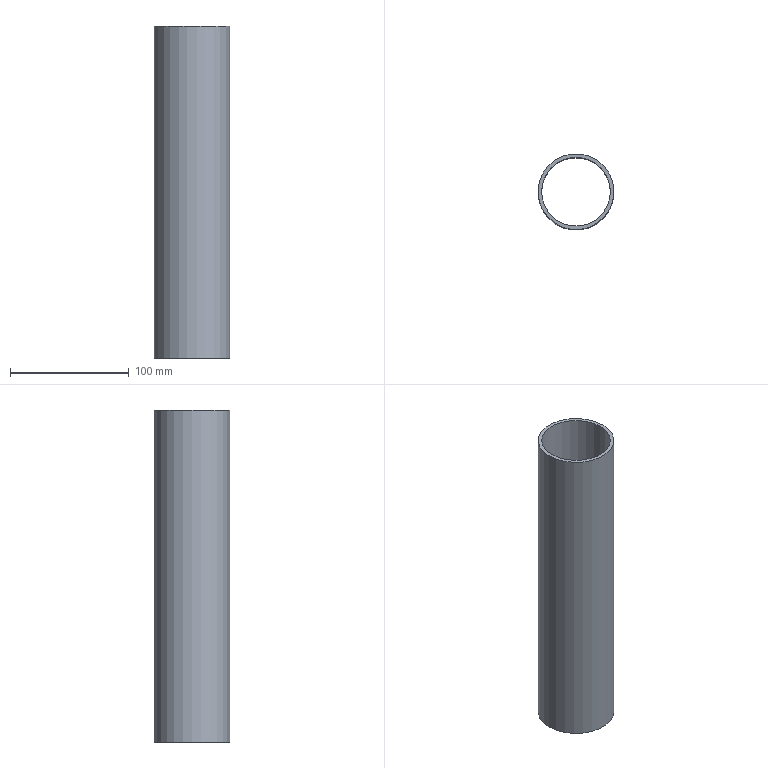Part | STEP file | JBJ-P-1000-06 | 1 solid | 4 faces | box 64 x 64 x 280 mm | volume 160975 mm3 | plane 2 | cylinder 2 | commonest cylinder face diameters 58 x1 64 x1
STEP:
#1=CARTESIAN_POINT('',(32.,0.,280.));
#2=VERTEX_POINT('',#1);
#3=CARTESIAN_POINT('',(0.,0.,280.));
#4=DIRECTION('',(0.,0.,1.));
#5=DIRECTION('',(1.,0.,0.));
#6=AXIS2_PLACEMENT_3D('',#3,#4,#5);
#7=CIRCLE('',#6,32.);
#8=EDGE_CURVE('',#2,#2,#7,.T.);
#9=ORIENTED_EDGE('',*,*,#8,.T.);
#10=EDGE_LOOP('',(#9));
#11=FACE_OUTER_BOUND('',#10,.T.);
#12=CARTESIAN_POINT('',(29.,0.,280.));
#13=VERTEX_POINT('',#12);
#14=CARTESIAN_POINT('',(0.,0.,280.));
#15=DIRECTION('',(0.,0.,1.));
#16=DIRECTION('',(1.,0.,0.));
#17=AXIS2_PLACEMENT_3D('',#14,#15,#16);
#18=CIRCLE('',#17,29.);
#19=EDGE_CURVE('',#13,#13,#18,.T.);
#20=ORIENTED_EDGE('',*,*,#19,.F.);
#21=EDGE_LOOP('',(#20));
#22=FACE_BOUND('',#21,.T.);
#23=CARTESIAN_POINT('',(0.,0.,280.));
#24=DIRECTION('',(0.,0.,1.));
#25=DIRECTION('',(1.,0.,0.));
#26=AXIS2_PLACEMENT_3D('',#23,#24,#25);
#27=PLANE('',#26);
#28=ADVANCED_FACE('',(#11,#22),#27,.T.);
#29=CARTESIAN_POINT('',(32.,0.,0.));
#30=VERTEX_POINT('',#29);
#31=CARTESIAN_POINT('',(0.,0.,0.));
#32=DIRECTION('',(0.,0.,1.));
#33=DIRECTION('',(1.,0.,0.));
#34=AXIS2_PLACEMENT_3D('',#31,#32,#33);
#35=CIRCLE('',#34,32.);
#36=EDGE_CURVE('',#30,#30,#35,.T.);
#37=ORIENTED_EDGE('',*,*,#36,.F.);
#38=EDGE_LOOP('',(#37));
#39=FACE_OUTER_BOUND('',#38,.T.);
#40=CARTESIAN_POINT('',(29.,0.,0.));
#41=VERTEX_POINT('',#40);
#42=CARTESIAN_POINT('',(0.,0.,0.));
#43=DIRECTION('',(0.,0.,1.));
#44=DIRECTION('',(1.,0.,0.));
#45=AXIS2_PLACEMENT_3D('',#42,#43,#44);
#46=CIRCLE('',#45,29.);
#47=EDGE_CURVE('',#41,#41,#46,.T.);
#48=ORIENTED_EDGE('',*,*,#47,.T.);
#49=EDGE_LOOP('',(#48));
#50=FACE_BOUND('',#49,.T.);
#51=CARTESIAN_POINT('',(0.,0.,0.));
#52=DIRECTION('',(0.,0.,1.));
#53=DIRECTION('',(1.,0.,0.));
#54=AXIS2_PLACEMENT_3D('',#51,#52,#53);
#55=PLANE('',#54);
#56=ADVANCED_FACE('',(#39,#50),#55,.F.);
#57=ORIENTED_EDGE('',*,*,#8,.F.);
#58=EDGE_LOOP('',(#57));
#59=FACE_OUTER_BOUND('',#58,.T.);
#60=ORIENTED_EDGE('',*,*,#36,.T.);
#61=EDGE_LOOP('',(#60));
#62=FACE_OUTER_BOUND('',#61,.T.);
#63=CARTESIAN_POINT('',(0.,0.,280.));
#64=DIRECTION('',(0.,0.,-1.));
#65=DIRECTION('',(-1.,0.,0.));
#66=AXIS2_PLACEMENT_3D('',#63,#64,#65);
#67=CYLINDRICAL_SURFACE('',#66,32.);
#68=ADVANCED_FACE('',(#59,#62),#67,.T.);
#69=ORIENTED_EDGE('',*,*,#19,.T.);
#70=EDGE_LOOP('',(#69));
#71=FACE_OUTER_BOUND('',#70,.T.);
#72=ORIENTED_EDGE('',*,*,#47,.F.);
#73=EDGE_LOOP('',(#72));
#74=FACE_OUTER_BOUND('',#73,.T.);
#75=CARTESIAN_POINT('',(0.,0.,280.));
#76=DIRECTION('',(0.,0.,-1.));
#77=DIRECTION('',(-1.,0.,0.));
#78=AXIS2_PLACEMENT_3D('',#75,#76,#77);
#79=CYLINDRICAL_SURFACE('',#78,29.);
#80=ADVANCED_FACE('',(#71,#74),#79,.F.);
#81=CLOSED_SHELL('',(#28,#56,#68,#80));
#82=MANIFOLD_SOLID_BREP('',#81);
#83=CARTESIAN_POINT('',(0.,0.,0.));
#84=DIRECTION('',(0.,0.,1.));
#85=DIRECTION('',(1.,0.,0.));
#86=AXIS2_PLACEMENT_3D('',#83,#84,#85);
#87=(LENGTH_UNIT()NAMED_UNIT(*)SI_UNIT(.MILLI.,.METRE.));
#88=UNCERTAINTY_MEASURE_WITH_UNIT(LENGTH_MEASURE(0.00001),#87,'','');
#89=(NAMED_UNIT(*)PLANE_ANGLE_UNIT()SI_UNIT($,.RADIAN.));
#90=(NAMED_UNIT(*)SI_UNIT($,.STERADIAN.)SOLID_ANGLE_UNIT());
#91=(GEOMETRIC_REPRESENTATION_CONTEXT(3)GLOBAL_UNCERTAINTY_ASSIGNED_CONTEXT((#88))GLOBAL_UNIT_ASSIGNED_CONTEXT((#87,#89,#90))REPRESENTATION_CONTEXT('',''));
#92=ADVANCED_BREP_SHAPE_REPRESENTATION('',(#82,#86),#91);